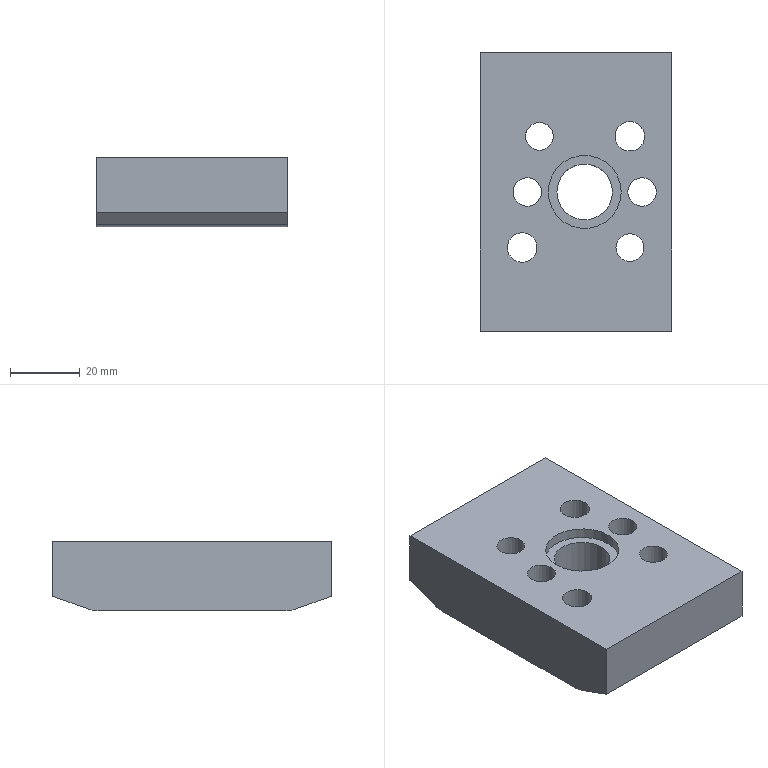Part | STEP file | lll_id3386_x_t | 1 solid | 23 faces | box 55 x 80 x 20 mm | volume 72093 mm3 | cylinder 12 | plane 11 | commonest cylinder face diameters 8 x2 8.2 x2 8.506 x2 14.507 x2 20 x2 16 x1
STEP:
#1=CARTESIAN_POINT('',(2682.,-16.,2.5));
#2=VERTEX_POINT('',#1);
#3=CARTESIAN_POINT('',(2686.,-16.,2.5));
#4=DIRECTION('',(0.,0.,-1.));
#5=DIRECTION('',(-1.,0.,0.));
#6=AXIS2_PLACEMENT_3D('',#3,#4,#5);
#7=CIRCLE('',#6,4.);
#8=EDGE_CURVE('',#2,#2,#7,.T.);
#9=ORIENTED_EDGE('',*,*,#8,.F.);
#10=EDGE_LOOP('',(#9));
#11=FACE_BOUND('',#10,.T.);
#12=CARTESIAN_POINT('',(2693.253,16.,2.5));
#13=VERTEX_POINT('',#12);
#14=CARTESIAN_POINT('',(2686.,16.,2.5));
#15=DIRECTION('',(0.,0.,1.));
#16=DIRECTION('',(1.,0.,0.));
#17=AXIS2_PLACEMENT_3D('',#14,#15,#16);
#18=CIRCLE('',#17,7.253);
#19=EDGE_CURVE('',#13,#13,#18,.T.);
#20=ORIENTED_EDGE('',*,*,#19,.T.);
#21=EDGE_LOOP('',(#20));
#22=FACE_BOUND('',#21,.T.);
#23=CARTESIAN_POINT('',(2698.,-26.737,2.5));
#24=VERTEX_POINT('',#23);
#25=CARTESIAN_POINT('',(2698.,26.737,2.5));
#26=VERTEX_POINT('',#25);
#27=CARTESIAN_POINT('',(2698.,0.,2.5));
#28=DIRECTION('',(0.,1.,0.));
#29=VECTOR('',#28,1.);
#30=LINE('',#27,#29);
#31=EDGE_CURVE('',#24,#26,#30,.T.);
#32=ORIENTED_EDGE('',*,*,#31,.F.);
#33=CARTESIAN_POINT('',(2643.,-26.737,2.5));
#34=VERTEX_POINT('',#33);
#35=CARTESIAN_POINT('',(2673.,-26.737,2.5));
#36=DIRECTION('',(-1.,0.,0.));
#37=VECTOR('',#36,1.);
#38=LINE('',#35,#37);
#39=EDGE_CURVE('',#24,#34,#38,.T.);
#40=ORIENTED_EDGE('',*,*,#39,.T.);
#41=CARTESIAN_POINT('',(2643.,26.737,2.5));
#42=VERTEX_POINT('',#41);
#43=CARTESIAN_POINT('',(2643.,0.,2.5));
#44=DIRECTION('',(0.,-1.,0.));
#45=VECTOR('',#44,1.);
#46=LINE('',#43,#45);
#47=EDGE_CURVE('',#42,#34,#46,.T.);
#48=ORIENTED_EDGE('',*,*,#47,.F.);
#49=CARTESIAN_POINT('',(2673.,26.737,2.5));
#50=DIRECTION('',(1.,0.,0.));
#51=VECTOR('',#50,1.);
#52=LINE('',#49,#51);
#53=EDGE_CURVE('',#42,#26,#52,.T.);
#54=ORIENTED_EDGE('',*,*,#53,.T.);
#55=EDGE_LOOP('',(#32,#40,#48,#54));
#56=FACE_BOUND('',#55,.T.);
#57=CARTESIAN_POINT('',(2652.4,0.,2.5));
#58=VERTEX_POINT('',#57);
#59=CARTESIAN_POINT('',(2656.5,0.,2.5));
#60=DIRECTION('',(0.,0.,-1.));
#61=DIRECTION('',(-1.,0.,0.));
#62=AXIS2_PLACEMENT_3D('',#59,#60,#61);
#63=CIRCLE('',#62,4.1);
#64=EDGE_CURVE('',#58,#58,#63,.T.);
#65=ORIENTED_EDGE('',*,*,#64,.F.);
#66=EDGE_LOOP('',(#65));
#67=FACE_BOUND('',#66,.T.);
#68=CARTESIAN_POINT('',(2685.4,0.,2.5));
#69=VERTEX_POINT('',#68);
#70=CARTESIAN_POINT('',(2689.5,0.,2.5));
#71=DIRECTION('',(0.,0.,-1.));
#72=DIRECTION('',(-1.,0.,0.));
#73=AXIS2_PLACEMENT_3D('',#70,#71,#72);
#74=CIRCLE('',#73,4.1);
#75=EDGE_CURVE('',#69,#69,#74,.T.);
#76=ORIENTED_EDGE('',*,*,#75,.F.);
#77=EDGE_LOOP('',(#76));
#78=FACE_BOUND('',#77,.T.);
#79=CARTESIAN_POINT('',(2681.,0.,2.5));
#80=VERTEX_POINT('',#79);
#81=CARTESIAN_POINT('',(2673.,0.,2.5));
#82=DIRECTION('',(0.,0.,1.));
#83=DIRECTION('',(1.,0.,0.));
#84=AXIS2_PLACEMENT_3D('',#81,#82,#83);
#85=CIRCLE('',#84,8.);
#86=EDGE_CURVE('',#80,#80,#85,.T.);
#87=ORIENTED_EDGE('',*,*,#86,.T.);
#88=EDGE_LOOP('',(#87));
#89=FACE_BOUND('',#88,.T.);
#90=CARTESIAN_POINT('',(2656.,16.,2.5));
#91=VERTEX_POINT('',#90);
#92=CARTESIAN_POINT('',(2660.,16.,2.5));
#93=DIRECTION('',(0.,0.,-1.));
#94=DIRECTION('',(-1.,0.,0.));
#95=AXIS2_PLACEMENT_3D('',#92,#93,#94);
#96=CIRCLE('',#95,4.);
#97=EDGE_CURVE('',#91,#91,#96,.T.);
#98=ORIENTED_EDGE('',*,*,#97,.F.);
#99=EDGE_LOOP('',(#98));
#100=FACE_BOUND('',#99,.T.);
#101=CARTESIAN_POINT('',(2662.253,-16.,2.5));
#102=VERTEX_POINT('',#101);
#103=CARTESIAN_POINT('',(2655.,-16.,2.5));
#104=DIRECTION('',(0.,0.,1.));
#105=DIRECTION('',(1.,0.,0.));
#106=AXIS2_PLACEMENT_3D('',#103,#104,#105);
#107=CIRCLE('',#106,7.253);
#108=EDGE_CURVE('',#102,#102,#107,.T.);
#109=ORIENTED_EDGE('',*,*,#108,.T.);
#110=EDGE_LOOP('',(#109));
#111=FACE_BOUND('',#110,.T.);
#112=CARTESIAN_POINT('',(2673.,0.,2.5));
#113=DIRECTION('',(0.,0.,-1.));
#114=DIRECTION('',(-1.,0.,0.));
#115=AXIS2_PLACEMENT_3D('',#112,#113,#114);
#116=PLANE('',#115);
#117=ADVANCED_FACE('',(#11,#22,#56,#67,#78,#89,#100,#111),#116,.T.);
#118=CARTESIAN_POINT('',(2643.,-40.,6.686));
#119=VERTEX_POINT('',#118);
#120=CARTESIAN_POINT('',(2643.,-40.,22.5));
#121=VERTEX_POINT('',#120);
#122=CARTESIAN_POINT('',(2643.,-40.,2.5));
#123=DIRECTION('',(0.,0.,1.));
#124=VECTOR('',#123,1.);
#125=LINE('',#122,#124);
#126=EDGE_CURVE('',#119,#121,#125,.T.);
#127=ORIENTED_EDGE('',*,*,#126,.F.);
#128=CARTESIAN_POINT('',(2698.,-40.,6.686));
#129=VERTEX_POINT('',#128);
#130=CARTESIAN_POINT('',(2673.,-40.,6.686));
#131=DIRECTION('',(1.,0.,0.));
#132=VECTOR('',#131,1.);
#133=LINE('',#130,#132);
#134=EDGE_CURVE('',#119,#129,#133,.T.);
#135=ORIENTED_EDGE('',*,*,#134,.T.);
#136=CARTESIAN_POINT('',(2698.,-40.,22.5));
#137=VERTEX_POINT('',#136);
#138=CARTESIAN_POINT('',(2698.,-40.,2.5));
#139=DIRECTION('',(0.,0.,1.));
#140=VECTOR('',#139,1.);
#141=LINE('',#138,#140);
#142=EDGE_CURVE('',#129,#137,#141,.T.);
#143=ORIENTED_EDGE('',*,*,#142,.T.);
#144=CARTESIAN_POINT('',(2673.,-40.,22.5));
#145=DIRECTION('',(-1.,0.,0.));
#146=VECTOR('',#145,1.);
#147=LINE('',#144,#146);
#148=EDGE_CURVE('',#137,#121,#147,.T.);
#149=ORIENTED_EDGE('',*,*,#148,.T.);
#150=EDGE_LOOP('',(#127,#135,#143,#149));
#151=FACE_OUTER_BOUND('',#150,.T.);
#152=CARTESIAN_POINT('',(2673.,-40.,2.5));
#153=DIRECTION('',(0.,-1.,0.));
#154=DIRECTION('',(0.,0.,-1.));
#155=AXIS2_PLACEMENT_3D('',#152,#153,#154);
#156=PLANE('',#155);
#157=ADVANCED_FACE('',(#151),#156,.T.);
#158=CARTESIAN_POINT('',(2698.,40.,6.686));
#159=VERTEX_POINT('',#158);
#160=CARTESIAN_POINT('',(2698.,40.,22.5));
#161=VERTEX_POINT('',#160);
#162=CARTESIAN_POINT('',(2698.,40.,2.5));
#163=DIRECTION('',(0.,0.,1.));
#164=VECTOR('',#163,1.);
#165=LINE('',#162,#164);
#166=EDGE_CURVE('',#159,#161,#165,.T.);
#167=ORIENTED_EDGE('',*,*,#166,.F.);
#168=CARTESIAN_POINT('',(2643.,40.,6.686));
#169=VERTEX_POINT('',#168);
#170=CARTESIAN_POINT('',(2673.,40.,6.686));
#171=DIRECTION('',(-1.,0.,0.));
#172=VECTOR('',#171,1.);
#173=LINE('',#170,#172);
#174=EDGE_CURVE('',#159,#169,#173,.T.);
#175=ORIENTED_EDGE('',*,*,#174,.T.);
#176=CARTESIAN_POINT('',(2643.,40.,22.5));
#177=VERTEX_POINT('',#176);
#178=CARTESIAN_POINT('',(2643.,40.,2.5));
#179=DIRECTION('',(0.,0.,1.));
#180=VECTOR('',#179,1.);
#181=LINE('',#178,#180);
#182=EDGE_CURVE('',#169,#177,#181,.T.);
#183=ORIENTED_EDGE('',*,*,#182,.T.);
#184=CARTESIAN_POINT('',(2673.,40.,22.5));
#185=DIRECTION('',(1.,0.,0.));
#186=VECTOR('',#185,1.);
#187=LINE('',#184,#186);
#188=EDGE_CURVE('',#177,#161,#187,.T.);
#189=ORIENTED_EDGE('',*,*,#188,.T.);
#190=EDGE_LOOP('',(#167,#175,#183,#189));
#191=FACE_OUTER_BOUND('',#190,.T.);
#192=CARTESIAN_POINT('',(2673.,40.,2.5));
#193=DIRECTION('',(0.,1.,0.));
#194=DIRECTION('',(0.,0.,1.));
#195=AXIS2_PLACEMENT_3D('',#192,#193,#194);
#196=PLANE('',#195);
#197=ADVANCED_FACE('',(#191),#196,.T.);
#198=CARTESIAN_POINT('',(2698.,-30.157,3.103));
#199=VERTEX_POINT('',#198);
#200=CARTESIAN_POINT('',(2698.,-3.334,-6.66));
#201=DIRECTION('',(0.,0.9397,-0.342));
#202=VECTOR('',#201,1.);
#203=LINE('',#200,#202);
#204=EDGE_CURVE('',#129,#199,#203,.T.);
#205=ORIENTED_EDGE('',*,*,#204,.T.);
#206=CARTESIAN_POINT('',(2698.,-26.737,12.5));
#207=DIRECTION('',(1.,0.,0.));
#208=DIRECTION('',(0.,0.,-1.));
#209=AXIS2_PLACEMENT_3D('',#206,#207,#208);
#210=CIRCLE('',#209,10.);
#211=EDGE_CURVE('',#199,#24,#210,.T.);
#212=ORIENTED_EDGE('',*,*,#211,.T.);
#213=ORIENTED_EDGE('',*,*,#31,.T.);
#214=CARTESIAN_POINT('',(2698.,30.157,3.103));
#215=VERTEX_POINT('',#214);
#216=CARTESIAN_POINT('',(2698.,26.737,12.5));
#217=DIRECTION('',(1.,0.,0.));
#218=DIRECTION('',(0.,0.,-1.));
#219=AXIS2_PLACEMENT_3D('',#216,#217,#218);
#220=CIRCLE('',#219,10.);
#221=EDGE_CURVE('',#26,#215,#220,.T.);
#222=ORIENTED_EDGE('',*,*,#221,.T.);
#223=CARTESIAN_POINT('',(2698.,3.334,-6.66));
#224=DIRECTION('',(0.,0.9397,0.342));
#225=VECTOR('',#224,1.);
#226=LINE('',#223,#225);
#227=EDGE_CURVE('',#215,#159,#226,.T.);
#228=ORIENTED_EDGE('',*,*,#227,.T.);
#229=ORIENTED_EDGE('',*,*,#166,.T.);
#230=CARTESIAN_POINT('',(2698.,0.,22.5));
#231=DIRECTION('',(0.,-1.,0.));
#232=VECTOR('',#231,1.);
#233=LINE('',#230,#232);
#234=EDGE_CURVE('',#161,#137,#233,.T.);
#235=ORIENTED_EDGE('',*,*,#234,.T.);
#236=ORIENTED_EDGE('',*,*,#142,.F.);
#237=EDGE_LOOP('',(#205,#212,#213,#222,#228,#229,#235,#236));
#238=FACE_OUTER_BOUND('',#237,.T.);
#239=CARTESIAN_POINT('',(2698.,0.,2.5));
#240=DIRECTION('',(1.,0.,0.));
#241=DIRECTION('',(0.,0.,-1.));
#242=AXIS2_PLACEMENT_3D('',#239,#240,#241);
#243=PLANE('',#242);
#244=ADVANCED_FACE('',(#238),#243,.T.);
#245=ORIENTED_EDGE('',*,*,#47,.T.);
#246=CARTESIAN_POINT('',(2643.,-30.157,3.103));
#247=VERTEX_POINT('',#246);
#248=CARTESIAN_POINT('',(2643.,-26.737,12.5));
#249=DIRECTION('',(-1.,0.,0.));
#250=DIRECTION('',(0.,0.,1.));
#251=AXIS2_PLACEMENT_3D('',#248,#249,#250);
#252=CIRCLE('',#251,10.);
#253=EDGE_CURVE('',#34,#247,#252,.T.);
#254=ORIENTED_EDGE('',*,*,#253,.T.);
#255=CARTESIAN_POINT('',(2643.,-3.334,-6.66));
#256=DIRECTION('',(0.,-0.9397,0.342));
#257=VECTOR('',#256,1.);
#258=LINE('',#255,#257);
#259=EDGE_CURVE('',#247,#119,#258,.T.);
#260=ORIENTED_EDGE('',*,*,#259,.T.);
#261=ORIENTED_EDGE('',*,*,#126,.T.);
#262=CARTESIAN_POINT('',(2643.,0.,22.5));
#263=DIRECTION('',(0.,1.,0.));
#264=VECTOR('',#263,1.);
#265=LINE('',#262,#264);
#266=EDGE_CURVE('',#121,#177,#265,.T.);
#267=ORIENTED_EDGE('',*,*,#266,.T.);
#268=ORIENTED_EDGE('',*,*,#182,.F.);
#269=CARTESIAN_POINT('',(2643.,30.157,3.103));
#270=VERTEX_POINT('',#269);
#271=CARTESIAN_POINT('',(2643.,3.334,-6.66));
#272=DIRECTION('',(0.,-0.9397,-0.342));
#273=VECTOR('',#272,1.);
#274=LINE('',#271,#273);
#275=EDGE_CURVE('',#169,#270,#274,.T.);
#276=ORIENTED_EDGE('',*,*,#275,.T.);
#277=CARTESIAN_POINT('',(2643.,26.737,12.5));
#278=DIRECTION('',(-1.,0.,0.));
#279=DIRECTION('',(0.,0.,1.));
#280=AXIS2_PLACEMENT_3D('',#277,#278,#279);
#281=CIRCLE('',#280,10.);
#282=EDGE_CURVE('',#270,#42,#281,.T.);
#283=ORIENTED_EDGE('',*,*,#282,.T.);
#284=EDGE_LOOP('',(#245,#254,#260,#261,#267,#268,#276,#283));
#285=FACE_OUTER_BOUND('',#284,.T.);
#286=CARTESIAN_POINT('',(2643.,0.,2.5));
#287=DIRECTION('',(-1.,0.,0.));
#288=DIRECTION('',(0.,0.,1.));
#289=AXIS2_PLACEMENT_3D('',#286,#287,#288);
#290=PLANE('',#289);
#291=ADVANCED_FACE('',(#285),#290,.T.);
#292=CARTESIAN_POINT('',(2690.,-16.,22.5));
#293=VERTEX_POINT('',#292);
#294=CARTESIAN_POINT('',(2686.,-16.,22.5));
#295=DIRECTION('',(0.,0.,1.));
#296=DIRECTION('',(1.,0.,0.));
#297=AXIS2_PLACEMENT_3D('',#294,#295,#296);
#298=CIRCLE('',#297,4.);
#299=EDGE_CURVE('',#293,#293,#298,.T.);
#300=ORIENTED_EDGE('',*,*,#299,.F.);
#301=EDGE_LOOP('',(#300));
#302=FACE_BOUND('',#301,.T.);
#303=CARTESIAN_POINT('',(2659.253,-16.,22.5));
#304=VERTEX_POINT('',#303);
#305=CARTESIAN_POINT('',(2655.,-16.,22.5));
#306=DIRECTION('',(0.,0.,1.));
#307=DIRECTION('',(1.,0.,0.));
#308=AXIS2_PLACEMENT_3D('',#305,#306,#307);
#309=CIRCLE('',#308,4.253);
#310=EDGE_CURVE('',#304,#304,#309,.T.);
#311=ORIENTED_EDGE('',*,*,#310,.F.);
#312=EDGE_LOOP('',(#311));
#313=FACE_BOUND('',#312,.T.);
#314=CARTESIAN_POINT('',(2664.,16.,22.5));
#315=VERTEX_POINT('',#314);
#316=CARTESIAN_POINT('',(2660.,16.,22.5));
#317=DIRECTION('',(0.,0.,1.));
#318=DIRECTION('',(1.,0.,0.));
#319=AXIS2_PLACEMENT_3D('',#316,#317,#318);
#320=CIRCLE('',#319,4.);
#321=EDGE_CURVE('',#315,#315,#320,.T.);
#322=ORIENTED_EDGE('',*,*,#321,.F.);
#323=EDGE_LOOP('',(#322));
#324=FACE_BOUND('',#323,.T.);
#325=CARTESIAN_POINT('',(2690.253,16.,22.5));
#326=VERTEX_POINT('',#325);
#327=CARTESIAN_POINT('',(2686.,16.,22.5));
#328=DIRECTION('',(0.,0.,1.));
#329=DIRECTION('',(1.,0.,0.));
#330=AXIS2_PLACEMENT_3D('',#327,#328,#329);
#331=CIRCLE('',#330,4.253);
#332=EDGE_CURVE('',#326,#326,#331,.T.);
#333=ORIENTED_EDGE('',*,*,#332,.F.);
#334=EDGE_LOOP('',(#333));
#335=FACE_BOUND('',#334,.T.);
#336=CARTESIAN_POINT('',(2662.5,0.,22.5));
#337=VERTEX_POINT('',#336);
#338=CARTESIAN_POINT('',(2673.,0.,22.5));
#339=DIRECTION('',(0.,0.,1.));
#340=DIRECTION('',(-1.,0.,0.));
#341=AXIS2_PLACEMENT_3D('',#338,#339,#340);
#342=CIRCLE('',#341,10.5);
#343=EDGE_CURVE('',#337,#337,#342,.T.);
#344=ORIENTED_EDGE('',*,*,#343,.F.);
#345=EDGE_LOOP('',(#344));
#346=FACE_BOUND('',#345,.T.);
#347=CARTESIAN_POINT('',(2693.6,0.,22.5));
#348=VERTEX_POINT('',#347);
#349=CARTESIAN_POINT('',(2689.5,0.,22.5));
#350=DIRECTION('',(0.,0.,1.));
#351=DIRECTION('',(1.,0.,0.));
#352=AXIS2_PLACEMENT_3D('',#349,#350,#351);
#353=CIRCLE('',#352,4.1);
#354=EDGE_CURVE('',#348,#348,#353,.T.);
#355=ORIENTED_EDGE('',*,*,#354,.F.);
#356=EDGE_LOOP('',(#355));
#357=FACE_BOUND('',#356,.T.);
#358=CARTESIAN_POINT('',(2660.6,0.,22.5));
#359=VERTEX_POINT('',#358);
#360=CARTESIAN_POINT('',(2656.5,0.,22.5));
#361=DIRECTION('',(0.,0.,1.));
#362=DIRECTION('',(1.,0.,0.));
#363=AXIS2_PLACEMENT_3D('',#360,#361,#362);
#364=CIRCLE('',#363,4.1);
#365=EDGE_CURVE('',#359,#359,#364,.T.);
#366=ORIENTED_EDGE('',*,*,#365,.F.);
#367=EDGE_LOOP('',(#366));
#368=FACE_BOUND('',#367,.T.);
#369=ORIENTED_EDGE('',*,*,#148,.F.);
#370=ORIENTED_EDGE('',*,*,#234,.F.);
#371=ORIENTED_EDGE('',*,*,#188,.F.);
#372=ORIENTED_EDGE('',*,*,#266,.F.);
#373=EDGE_LOOP('',(#369,#370,#371,#372));
#374=FACE_BOUND('',#373,.T.);
#375=CARTESIAN_POINT('',(2673.,0.,22.5));
#376=DIRECTION('',(0.,0.,1.));
#377=DIRECTION('',(1.,0.,0.));
#378=AXIS2_PLACEMENT_3D('',#375,#376,#377);
#379=PLANE('',#378);
#380=ADVANCED_FACE('',(#302,#313,#324,#335,#346,#357,#368,#374),#379,.T.);
#381=ORIENTED_EDGE('',*,*,#64,.T.);
#382=EDGE_LOOP('',(#381));
#383=FACE_BOUND('',#382,.T.);
#384=ORIENTED_EDGE('',*,*,#365,.T.);
#385=EDGE_LOOP('',(#384));
#386=FACE_BOUND('',#385,.T.);
#387=CARTESIAN_POINT('',(2656.5,0.,-2.5));
#388=DIRECTION('',(0.,0.,1.));
#389=DIRECTION('',(1.,0.,0.));
#390=AXIS2_PLACEMENT_3D('',#387,#388,#389);
#391=CYLINDRICAL_SURFACE('',#390,4.1);
#392=ADVANCED_FACE('',(#383,#386),#391,.F.);
#393=ORIENTED_EDGE('',*,*,#75,.T.);
#394=EDGE_LOOP('',(#393));
#395=FACE_BOUND('',#394,.T.);
#396=ORIENTED_EDGE('',*,*,#354,.T.);
#397=EDGE_LOOP('',(#396));
#398=FACE_BOUND('',#397,.T.);
#399=CARTESIAN_POINT('',(2689.5,0.,-2.5));
#400=DIRECTION('',(0.,0.,1.));
#401=DIRECTION('',(1.,0.,0.));
#402=AXIS2_PLACEMENT_3D('',#399,#400,#401);
#403=CYLINDRICAL_SURFACE('',#402,4.1);
#404=ADVANCED_FACE('',(#395,#398),#403,.F.);
#405=CARTESIAN_POINT('',(2662.5,0.,19.5));
#406=VERTEX_POINT('',#405);
#407=CARTESIAN_POINT('',(2673.,0.,19.5));
#408=DIRECTION('',(0.,0.,1.));
#409=DIRECTION('',(-1.,0.,0.));
#410=AXIS2_PLACEMENT_3D('',#407,#408,#409);
#411=CIRCLE('',#410,10.5);
#412=EDGE_CURVE('',#406,#406,#411,.T.);
#413=ORIENTED_EDGE('',*,*,#412,.T.);
#414=EDGE_LOOP('',(#413));
#415=FACE_BOUND('',#414,.T.);
#416=CARTESIAN_POINT('',(2665.,0.,19.5));
#417=VERTEX_POINT('',#416);
#418=CARTESIAN_POINT('',(2673.,0.,19.5));
#419=DIRECTION('',(0.,0.,-1.));
#420=DIRECTION('',(-1.,0.,0.));
#421=AXIS2_PLACEMENT_3D('',#418,#419,#420);
#422=CIRCLE('',#421,8.);
#423=EDGE_CURVE('',#417,#417,#422,.T.);
#424=ORIENTED_EDGE('',*,*,#423,.T.);
#425=EDGE_LOOP('',(#424));
#426=FACE_BOUND('',#425,.T.);
#427=CARTESIAN_POINT('',(2673.,0.,19.5));
#428=DIRECTION('',(0.,0.,-1.));
#429=DIRECTION('',(0.,-1.,0.));
#430=AXIS2_PLACEMENT_3D('',#427,#428,#429);
#431=PLANE('',#430);
#432=ADVANCED_FACE('',(#415,#426),#431,.F.);
#433=ORIENTED_EDGE('',*,*,#343,.T.);
#434=EDGE_LOOP('',(#433));
#435=FACE_BOUND('',#434,.T.);
#436=ORIENTED_EDGE('',*,*,#412,.F.);
#437=EDGE_LOOP('',(#436));
#438=FACE_BOUND('',#437,.T.);
#439=CARTESIAN_POINT('',(2673.,0.,19.5));
#440=DIRECTION('',(0.,0.,-1.));
#441=DIRECTION('',(0.,-1.,0.));
#442=AXIS2_PLACEMENT_3D('',#439,#440,#441);
#443=CYLINDRICAL_SURFACE('',#442,10.5);
#444=ADVANCED_FACE('',(#435,#438),#443,.F.);
#445=ORIENTED_EDGE('',*,*,#86,.F.);
#446=EDGE_LOOP('',(#445));
#447=FACE_BOUND('',#446,.T.);
#448=ORIENTED_EDGE('',*,*,#423,.F.);
#449=EDGE_LOOP('',(#448));
#450=FACE_BOUND('',#449,.T.);
#451=CARTESIAN_POINT('',(2673.,0.,20.5));
#452=DIRECTION('',(0.,0.,-1.));
#453=DIRECTION('',(0.,-1.,0.));
#454=AXIS2_PLACEMENT_3D('',#451,#452,#453);
#455=CYLINDRICAL_SURFACE('',#454,8.);
#456=ADVANCED_FACE('',(#447,#450),#455,.F.);
#457=ORIENTED_EDGE('',*,*,#259,.F.);
#458=CARTESIAN_POINT('',(2732.61,-30.157,3.103));
#459=DIRECTION('',(1.,0.,0.));
#460=VECTOR('',#459,1.);
#461=LINE('',#458,#460);
#462=EDGE_CURVE('',#247,#199,#461,.T.);
#463=ORIENTED_EDGE('',*,*,#462,.T.);
#464=ORIENTED_EDGE('',*,*,#204,.F.);
#465=ORIENTED_EDGE('',*,*,#134,.F.);
#466=EDGE_LOOP('',(#457,#463,#464,#465));
#467=FACE_OUTER_BOUND('',#466,.T.);
#468=CARTESIAN_POINT('',(2732.61,-122.996,36.894));
#469=DIRECTION('',(0.,0.342,0.9397));
#470=DIRECTION('',(0.,0.9397,-0.342));
#471=AXIS2_PLACEMENT_3D('',#468,#469,#470);
#472=PLANE('',#471);
#473=ADVANCED_FACE('',(#467),#472,.F.);
#474=ORIENTED_EDGE('',*,*,#227,.F.);
#475=CARTESIAN_POINT('',(2732.617,30.157,3.103));
#476=DIRECTION('',(-1.,0.,0.));
#477=VECTOR('',#476,1.);
#478=LINE('',#475,#477);
#479=EDGE_CURVE('',#215,#270,#478,.T.);
#480=ORIENTED_EDGE('',*,*,#479,.T.);
#481=ORIENTED_EDGE('',*,*,#275,.F.);
#482=ORIENTED_EDGE('',*,*,#174,.F.);
#483=EDGE_LOOP('',(#474,#480,#481,#482));
#484=FACE_OUTER_BOUND('',#483,.T.);
#485=CARTESIAN_POINT('',(2732.617,122.985,36.89));
#486=DIRECTION('',(0.,-0.342,0.9397));
#487=DIRECTION('',(0.,0.9397,0.342));
#488=AXIS2_PLACEMENT_3D('',#485,#486,#487);
#489=PLANE('',#488);
#490=ADVANCED_FACE('',(#484),#489,.F.);
#491=ORIENTED_EDGE('',*,*,#211,.F.);
#492=ORIENTED_EDGE('',*,*,#462,.F.);
#493=ORIENTED_EDGE('',*,*,#253,.F.);
#494=ORIENTED_EDGE('',*,*,#39,.F.);
#495=EDGE_LOOP('',(#491,#492,#493,#494));
#496=FACE_OUTER_BOUND('',#495,.T.);
#497=CARTESIAN_POINT('',(2673.,-26.737,12.5));
#498=DIRECTION('',(1.,0.,0.));
#499=DIRECTION('',(0.,0.,-1.));
#500=AXIS2_PLACEMENT_3D('',#497,#498,#499);
#501=CYLINDRICAL_SURFACE('',#500,10.);
#502=ADVANCED_FACE('',(#496),#501,.T.);
#503=ORIENTED_EDGE('',*,*,#282,.F.);
#504=ORIENTED_EDGE('',*,*,#479,.F.);
#505=ORIENTED_EDGE('',*,*,#221,.F.);
#506=ORIENTED_EDGE('',*,*,#53,.F.);
#507=EDGE_LOOP('',(#503,#504,#505,#506));
#508=FACE_OUTER_BOUND('',#507,.T.);
#509=CARTESIAN_POINT('',(2673.,26.737,12.5));
#510=DIRECTION('',(-1.,0.,0.));
#511=DIRECTION('',(0.,-1.,0.));
#512=AXIS2_PLACEMENT_3D('',#509,#510,#511);
#513=CYLINDRICAL_SURFACE('',#512,10.);
#514=ADVANCED_FACE('',(#508),#513,.T.);
#515=ORIENTED_EDGE('',*,*,#332,.T.);
#516=EDGE_LOOP('',(#515));
#517=FACE_BOUND('',#516,.T.);
#518=CARTESIAN_POINT('',(2690.253,16.,13.5));
#519=VERTEX_POINT('',#518);
#520=CARTESIAN_POINT('',(2686.,16.,13.5));
#521=DIRECTION('',(0.,0.,1.));
#522=DIRECTION('',(1.,0.,0.));
#523=AXIS2_PLACEMENT_3D('',#520,#521,#522);
#524=CIRCLE('',#523,4.253);
#525=EDGE_CURVE('',#519,#519,#524,.T.);
#526=ORIENTED_EDGE('',*,*,#525,.F.);
#527=EDGE_LOOP('',(#526));
#528=FACE_BOUND('',#527,.T.);
#529=CARTESIAN_POINT('',(2686.,16.,-2.5));
#530=DIRECTION('',(0.,0.,1.));
#531=DIRECTION('',(1.,0.,0.));
#532=AXIS2_PLACEMENT_3D('',#529,#530,#531);
#533=CYLINDRICAL_SURFACE('',#532,4.253);
#534=ADVANCED_FACE('',(#517,#528),#533,.F.);
#535=ORIENTED_EDGE('',*,*,#525,.T.);
#536=EDGE_LOOP('',(#535));
#537=FACE_BOUND('',#536,.T.);
#538=CARTESIAN_POINT('',(2693.253,16.,13.5));
#539=VERTEX_POINT('',#538);
#540=CARTESIAN_POINT('',(2686.,16.,13.5));
#541=DIRECTION('',(0.,0.,1.));
#542=DIRECTION('',(1.,0.,0.));
#543=AXIS2_PLACEMENT_3D('',#540,#541,#542);
#544=CIRCLE('',#543,7.253);
#545=EDGE_CURVE('',#539,#539,#544,.T.);
#546=ORIENTED_EDGE('',*,*,#545,.F.);
#547=EDGE_LOOP('',(#546));
#548=FACE_BOUND('',#547,.T.);
#549=CARTESIAN_POINT('',(2686.,16.,13.5));
#550=DIRECTION('',(0.,0.,1.));
#551=DIRECTION('',(1.,0.,0.));
#552=AXIS2_PLACEMENT_3D('',#549,#550,#551);
#553=PLANE('',#552);
#554=ADVANCED_FACE('',(#537,#548),#553,.F.);
#555=ORIENTED_EDGE('',*,*,#545,.T.);
#556=EDGE_LOOP('',(#555));
#557=FACE_BOUND('',#556,.T.);
#558=ORIENTED_EDGE('',*,*,#19,.F.);
#559=EDGE_LOOP('',(#558));
#560=FACE_BOUND('',#559,.T.);
#561=CARTESIAN_POINT('',(2686.,16.,2.5));
#562=DIRECTION('',(0.,0.,1.));
#563=DIRECTION('',(1.,0.,0.));
#564=AXIS2_PLACEMENT_3D('',#561,#562,#563);
#565=CYLINDRICAL_SURFACE('',#564,7.253);
#566=ADVANCED_FACE('',(#557,#560),#565,.F.);
#567=ORIENTED_EDGE('',*,*,#97,.T.);
#568=EDGE_LOOP('',(#567));
#569=FACE_BOUND('',#568,.T.);
#570=ORIENTED_EDGE('',*,*,#321,.T.);
#571=EDGE_LOOP('',(#570));
#572=FACE_BOUND('',#571,.T.);
#573=CARTESIAN_POINT('',(2660.,16.,-2.5));
#574=DIRECTION('',(0.,0.,1.));
#575=DIRECTION('',(1.,0.,0.));
#576=AXIS2_PLACEMENT_3D('',#573,#574,#575);
#577=CYLINDRICAL_SURFACE('',#576,4.);
#578=ADVANCED_FACE('',(#569,#572),#577,.F.);
#579=ORIENTED_EDGE('',*,*,#310,.T.);
#580=EDGE_LOOP('',(#579));
#581=FACE_BOUND('',#580,.T.);
#582=CARTESIAN_POINT('',(2659.253,-16.,13.5));
#583=VERTEX_POINT('',#582);
#584=CARTESIAN_POINT('',(2655.,-16.,13.5));
#585=DIRECTION('',(0.,0.,1.));
#586=DIRECTION('',(1.,0.,0.));
#587=AXIS2_PLACEMENT_3D('',#584,#585,#586);
#588=CIRCLE('',#587,4.253);
#589=EDGE_CURVE('',#583,#583,#588,.T.);
#590=ORIENTED_EDGE('',*,*,#589,.F.);
#591=EDGE_LOOP('',(#590));
#592=FACE_BOUND('',#591,.T.);
#593=CARTESIAN_POINT('',(2655.,-16.,-2.5));
#594=DIRECTION('',(0.,0.,1.));
#595=DIRECTION('',(1.,0.,0.));
#596=AXIS2_PLACEMENT_3D('',#593,#594,#595);
#597=CYLINDRICAL_SURFACE('',#596,4.253);
#598=ADVANCED_FACE('',(#581,#592),#597,.F.);
#599=ORIENTED_EDGE('',*,*,#589,.T.);
#600=EDGE_LOOP('',(#599));
#601=FACE_BOUND('',#600,.T.);
#602=CARTESIAN_POINT('',(2662.253,-16.,13.5));
#603=VERTEX_POINT('',#602);
#604=CARTESIAN_POINT('',(2655.,-16.,13.5));
#605=DIRECTION('',(0.,0.,1.));
#606=DIRECTION('',(1.,0.,0.));
#607=AXIS2_PLACEMENT_3D('',#604,#605,#606);
#608=CIRCLE('',#607,7.253);
#609=EDGE_CURVE('',#603,#603,#608,.T.);
#610=ORIENTED_EDGE('',*,*,#609,.F.);
#611=EDGE_LOOP('',(#610));
#612=FACE_BOUND('',#611,.T.);
#613=CARTESIAN_POINT('',(2655.,-16.,13.5));
#614=DIRECTION('',(0.,0.,1.));
#615=DIRECTION('',(1.,0.,0.));
#616=AXIS2_PLACEMENT_3D('',#613,#614,#615);
#617=PLANE('',#616);
#618=ADVANCED_FACE('',(#601,#612),#617,.F.);
#619=ORIENTED_EDGE('',*,*,#609,.T.);
#620=EDGE_LOOP('',(#619));
#621=FACE_BOUND('',#620,.T.);
#622=ORIENTED_EDGE('',*,*,#108,.F.);
#623=EDGE_LOOP('',(#622));
#624=FACE_BOUND('',#623,.T.);
#625=CARTESIAN_POINT('',(2655.,-16.,2.5));
#626=DIRECTION('',(0.,0.,1.));
#627=DIRECTION('',(1.,0.,0.));
#628=AXIS2_PLACEMENT_3D('',#625,#626,#627);
#629=CYLINDRICAL_SURFACE('',#628,7.253);
#630=ADVANCED_FACE('',(#621,#624),#629,.F.);
#631=ORIENTED_EDGE('',*,*,#8,.T.);
#632=EDGE_LOOP('',(#631));
#633=FACE_BOUND('',#632,.T.);
#634=ORIENTED_EDGE('',*,*,#299,.T.);
#635=EDGE_LOOP('',(#634));
#636=FACE_BOUND('',#635,.T.);
#637=CARTESIAN_POINT('',(2686.,-16.,-2.5));
#638=DIRECTION('',(0.,0.,1.));
#639=DIRECTION('',(1.,0.,0.));
#640=AXIS2_PLACEMENT_3D('',#637,#638,#639);
#641=CYLINDRICAL_SURFACE('',#640,4.);
#642=ADVANCED_FACE('',(#633,#636),#641,.F.);
#643=CLOSED_SHELL('',(#117,#157,#197,#244,#291,#380,#392,#404,#432,#444,#456,#473,#490,#502,#514,#534,#554,#566,#578,#598,#618,#630,#642));
#644=MANIFOLD_SOLID_BREP('',#643);
#645=(LENGTH_UNIT()NAMED_UNIT(*)SI_UNIT(.MILLI.,.METRE.));
#646=UNCERTAINTY_MEASURE_WITH_UNIT(LENGTH_MEASURE(0.00002),#645,'','');
#647=(NAMED_UNIT(*)PLANE_ANGLE_UNIT()SI_UNIT($,.RADIAN.));
#648=PLANE_ANGLE_MEASURE_WITH_UNIT(PLANE_ANGLE_MEASURE(0.01745),#647);
#649=DIMENSIONAL_EXPONENTS(0.,0.,0.,0.,0.,0.,0.);
#650=(CONVERSION_BASED_UNIT('DEGREE',#648)NAMED_UNIT(#649)PLANE_ANGLE_UNIT());
#651=(NAMED_UNIT(*)SI_UNIT($,.STERADIAN.)SOLID_ANGLE_UNIT());
#652=(GEOMETRIC_REPRESENTATION_CONTEXT(3)GLOBAL_UNCERTAINTY_ASSIGNED_CONTEXT((#646))GLOBAL_UNIT_ASSIGNED_CONTEXT((#645,#650,#651))REPRESENTATION_CONTEXT('',''));
#653=ADVANCED_BREP_SHAPE_REPRESENTATION('',(#644),#652);